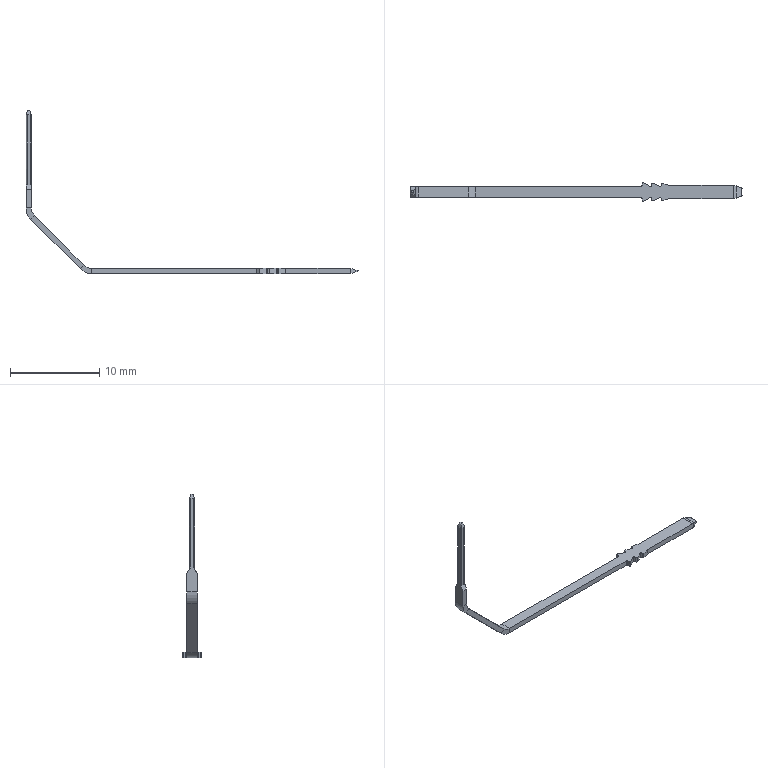Part | NX | features BREP 1 | 1 solid | 77 faces | box 37.2 x 2.1 x 18.3 mm | volume 35.308 mm3 | plane 44 | cylinder 33 | commonest cylinder face diameters 0.3 x12 0.2 x9 0.04 x4 0.025 x2 2 x2 2.4 x2